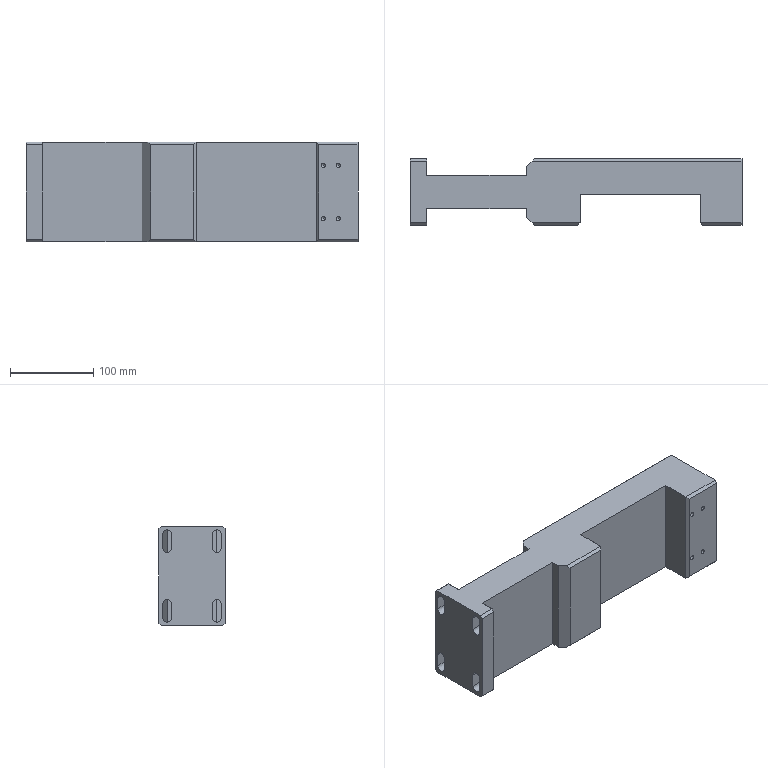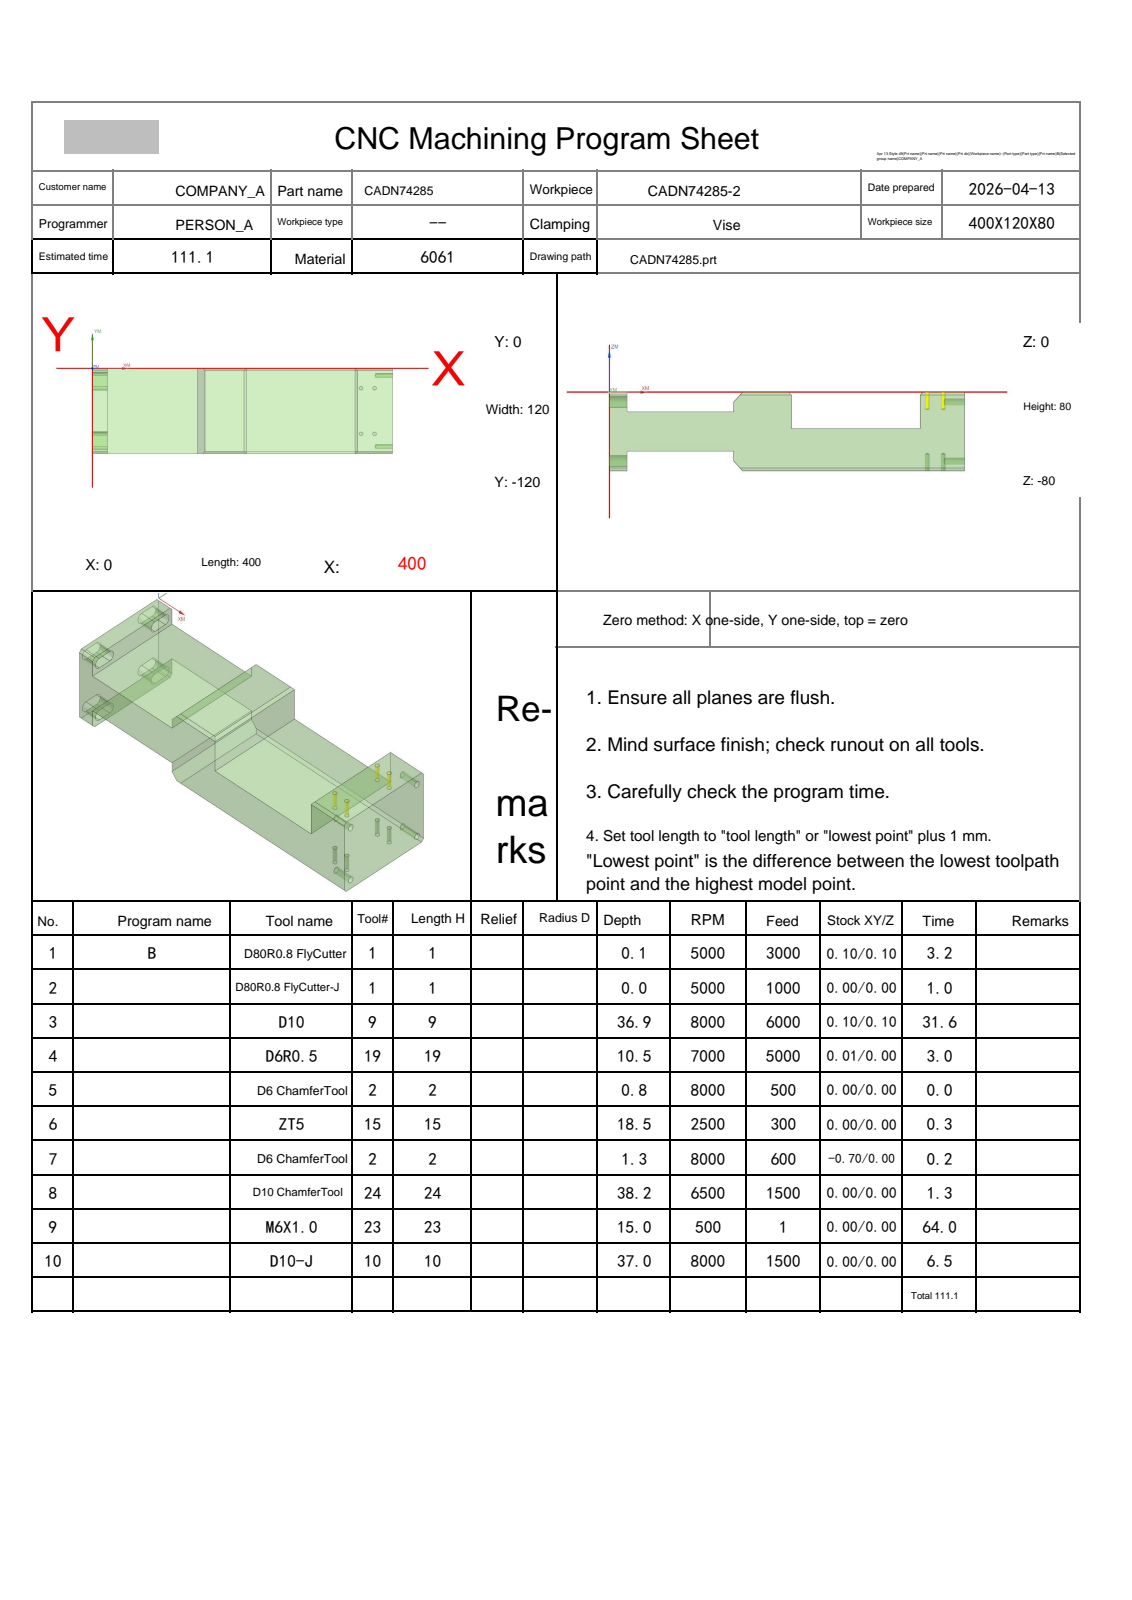NC program | NX | posted by the shop | part box 400 x 80 x 120 mm
Lines 148 to 1262 of 11018:
N3 T09 M06
(D10  D=10. R=0. H=09 ce=0.10 di=0.10)
G00 G90 G54 X281.7 Y-134.5 M03 S8000
G43 H09 Z14.8
M08
Z.404
G01 Z-.796 F6000.
Y-127.08
G03 X274.7 Y-120.08 I-7. J0.0
G01 X210.176
G02 X209.144 Y-123. I-5.292 J.229
G01 X206.806
G02 X202.867 Y-124.337 I-3.939 J5.133
G01 X149.133
G02 X145.194 Y-123. I0.0 J6.471
G01 X142.86
G02 X142.513 Y-122.469 I4.246 J3.15
G01 X142.281 Y-122.023
X142.117 Y-121.559
X141.891 Y-120.662
X141.789 Y-120.08
X135.073
X135.144 Y-120.637
X135.177 Y-120.857
X135.243 Y-121.187
X135.332 Y-121.516
X135.446 Y-121.845
X135.586 Y-122.175
X135.756 Y-122.504
X135.888 Y-122.723
X136.081 Y-123.
X135.852
G02 X134.823 Y-120.08 I4.186 J3.116
G01 X26.095
X25.178
G02 X24.433 Y-122.58 I-5.192 J.186
X24.15 Y-123. I-4.447 J2.686
G01 X23.935
G02 X20. Y-124.337 I-3.956 J5.184
G01 X.08
Y-123.
X.026
Y-124.337
X0.0
Y-123.
X-.08
Y-122.937
X-.001
X0.0 Y-122.938
X.026 Y-122.937
X.027
X.08 Y-122.938
X20. Y-122.937
G03 X25.1 Y-117.817 I-.021 J5.121
G01 Y-117.796
Y-2.204
Y-2.183
G03 X20. Y2.937 I-5.121 J0.0
G01 X.08
X-.08
Y3.
X.08
Y4.337
X20.006
G02 X23.935 Y3. I-.026 J-6.521
G01 X24.15
G02 X25.178 Y.08 I-4.164 J-3.106
G01 X134.824
G02 X135.861 Y3. I5.378 J-.266
G01 X136.079
X135.912 Y2.761
X135.787 Y2.557
X135.696 Y2.395
X135.535 Y2.064
X135.405 Y1.736
X135.284 Y1.351
X135.197 Y.967
X135.144 Y.637
X135.077 Y.11
X135.215 Y.08
X138.463
G02 X139.404 Y-.583 I0.0 J-1.
G01 X141.485 Y-6.408
G03 X142.044 Y-6.995 I.941 J.337
G02 X142.663 Y-7.915 I-.381 J-.924
G01 Y-112.085
G02 X141.667 Y-113.08 I-1. J.005
G01 X135.073
X134.952 Y-113.081
X134.823 Y-113.08
X33.095
G02 X32.1 Y-112.085 I.005 J1.
G01 Y-7.915
G02 X33.095 Y-6.92 I1. J-.005
G01 X39.1
X134.468
X138.169
G02 X138.868 Y-7.62 I0.0 J-.7
X138.826 Y-7.859 I-.7 J0.0
G01 X135.722 Y-16.404
G03 X135.663 Y-16.744 I.94 J-.341
G01 Y-105.085
G02 X134.668 Y-106.08 I-1. J.005
G01 X40.095
G02 X39.1 Y-105.085 I.005 J1.
G01 Y-14.915
G02 X40.095 Y-13.92 I1. J-.005
G01 X131.967
G02 X132.567 Y-14.52 I-.001 J-.6
X132.517 Y-14.759 I-.6 J0.0
G01 X128.745 Y-23.438
G03 X128.663 Y-23.836 I.917 J-.398
G01 Y-98.086
G02 X127.668 Y-99.08 I-1. J.006
G01 X47.094
G02 X46.1 Y-98.086 I.006 J1.
G01 Y-21.914
G02 X47.094 Y-20.92 I1. J-.006
G01 X125.022
G02 X125.622 Y-21.52 I-.001 J-.6
X125.571 Y-21.761 I-.6 J0.0
G01 X121.747 Y-30.442
G03 X121.663 Y-30.844 I.915 J-.403
G01 Y-91.086
G02 X120.668 Y-92.08 I-1. J.006
G01 X54.094
G02 X53.1 Y-91.086 I.006 J1.
G01 Y-28.914
G02 X54.094 Y-27.92 I1. J-.006
G01 X118.027
G02 X118.627 Y-28.52 I0.0 J-.6
X118.576 Y-28.762 I-.6 J0.0
G01 X114.747 Y-37.442
G03 X114.663 Y-37.845 I.915 J-.403
G01 Y-84.086
G02 X113.668 Y-85.08 I-1. J.006
G01 X61.094
G02 X60.1 Y-84.086 I.006 J1.
G01 Y-35.914
G02 X61.094 Y-34.92 I1. J-.006
G01 X111.028
G02 X111.627 Y-35.52 I0.0 J-.6
X111.577 Y-35.762 I-.6 J0.0
G01 X107.747 Y-44.442
G03 X107.663 Y-44.845 I.915 J-.403
G01 Y-77.086
G02 X106.668 Y-78.08 I-1. J.006
G01 X68.094
G02 X67.1 Y-77.086 I.006 J1.
G01 Y-42.914
G02 X68.094 Y-41.92 I1. J-.006
G01 X104.028
G02 X104.628 Y-42.52 I0.0 J-.6
X104.577 Y-42.762 I-.6 J0.0
G01 X100.747 Y-51.442
G03 X100.663 Y-51.845 I.915 J-.403
G01 Y-70.086
G02 X99.669 Y-71.08 I-1. J.006
G01 X75.094
G02 X74.1 Y-70.086 I.006 J1.
G01 Y-49.914
G02 X75.094 Y-48.92 I1. J-.006
G01 X97.028
G02 X97.628 Y-49.52 I0.0 J-.6
X97.577 Y-49.762 I-.6 J0.0
G01 X93.748 Y-58.442
G03 X93.663 Y-58.845 I.915 J-.403
G01 Y-63.086
G02 X92.669 Y-64.08 I-1. J.006
G01 X82.094
G02 X81.1 Y-63.086 I.006 J1.
G01 Y-56.914
G02 X82.094 Y-55.92 I1. J-.006
G01 X90.629
G03 X91.208 Y-55.735 I-.001 J1.
G01 X100.302 Y-49.261
X100.428 Y-49.154
X107.37 Y-42.213
X114.37 Y-35.213
X121.369 Y-28.212
X128.364 Y-21.21
X128.367 Y-21.207
X135.301 Y-14.189
X135.341 Y-14.146
X141.451 Y-7.167
G03 X141.695 Y-6.593 I-.753 J.658
G01 X142.433 Y2.115
G02 X142.544 Y2.477 I.897 J-.077
X142.877 Y3. I4.8 J-2.683
G01 X145.194
G02 X149.133 Y4.337 I3.939 J-5.134
G01 X202.867
G02 X206.806 Y3. I0.0 J-6.471
G01 X209.099
G02 X210.187 Y.08 I-4.43 J-3.314
G01 X344.823
G02 X345.85 Y3. I5.198 J-.188
G01 X348.194
G02 X352.133 Y4.337 I3.939 J-5.133
G01 X399.92
Y3.
X400.08
Y2.937
X399.92 Y2.938
X352.133 Y2.937
G03 X347.063 Y-2.133 I0.0 J-5.071
G01 Y-117.867
G03 X352.133 Y-122.937 I5.071 J0.0
G01 X400.
X400.001
X400.08
Y-123.
X400.
Y-124.337
X352.133
G02 X348.194 Y-123. I0.0 J6.471
G01 X345.865
G02 X344.824 Y-120.08 I4.252 J3.162
G01 X277.714
G02 X276.901 Y-119.662 I.001 J1.
G01 X272.499 Y-113.498
G03 X271.686 Y-113.08 I-.813 J-.582
G01 X210.333
G02 X209.337 Y-112.085 I.005 J1.
G01 Y-8.407
G03 X208.893 Y-7.704 I-.779 J-.001
G01 X208.537 Y-7.536
X208.357 Y-7.495
G03 X207.937 Y-7.915 I0.0 J-.42
G01 Y-117.867
G02 X202.867 Y-122.937 I-5.071 J0.0
G01 X149.133
G02 X144.063 Y-117.867 I0.0 J5.071
G01 Y-2.133
G02 X149.133 Y2.937 I5.071 J0.0
G01 X202.867
G02 X207.937 Y-2.133 I0.0 J-5.071
G01 Y-7.915
G03 X208.357 Y-8.335 I.42 J0.0
G01 X208.537 Y-8.295
X209.136 Y-8.011
G03 X209.356 Y-7.727 I-.172 J.361
G02 X210.333 Y-6.92 I.981 J-.193
G01 X339.067
G02 X340.063 Y-7.915 I-.005 J-1.
G01 Y-112.085
G02 X339.067 Y-113.08 I-1. J.005
G01 X277.714
G02 X276.901 Y-112.662 I.001 J1.
G01 X272.499 Y-106.498
G03 X271.686 Y-106.08 I-.813 J-.582
G01 X217.332
G02 X216.337 Y-105.085 I.005 J1.
G01 Y-14.915
G02 X217.332 Y-13.92 I1. J-.005
G01 X332.068
G02 X333.063 Y-14.915 I-.005 J-1.
G01 Y-105.085
G02 X332.068 Y-106.08 I-1. J.005
G01 X277.714
G02 X276.901 Y-105.662 I.001 J1.
G01 X272.499 Y-99.498
G03 X271.686 Y-99.08 I-.813 J-.582
G01 X224.332
G02 X223.337 Y-98.086 I.006 J1.
G01 Y-21.914
G02 X224.332 Y-20.92 I1. J-.006
G01 X325.068
G02 X326.063 Y-21.914 I-.006 J-1.
G01 Y-98.086
G02 X325.068 Y-99.08 I-1. J.006
G01 X277.714
G02 X276.901 Y-98.662 I.001 J1.
G01 X272.499 Y-92.498
G03 X271.686 Y-92.08 I-.813 J-.582
G01 X231.332
G02 X230.337 Y-91.086 I.006 J1.
G01 Y-28.914
G02 X231.332 Y-27.92 I1. J-.006
G01 X318.068
G02 X319.063 Y-28.914 I-.006 J-1.
G01 Y-91.086
G02 X318.068 Y-92.08 I-1. J.006
G01 X277.714
G02 X276.901 Y-91.662 I.001 J1.
G01 X272.499 Y-85.498
G03 X271.686 Y-85.08 I-.813 J-.582
G01 X238.331
G02 X237.337 Y-84.086 I.006 J1.
G01 Y-35.914
G02 X238.331 Y-34.92 I1. J-.006
G01 X311.069
G02 X312.063 Y-35.914 I-.006 J-1.
G01 Y-84.086
G02 X311.069 Y-85.08 I-1. J.006
G01 X277.714
G02 X276.901 Y-84.662 I0.0 J1.
G01 X272.499 Y-78.498
G03 X271.686 Y-78.08 I-.813 J-.582
G01 X245.331
G02 X244.337 Y-77.086 I.006 J1.
G01 Y-42.914
G02 X245.331 Y-41.92 I1. J-.006
G01 X304.069
G02 X305.063 Y-42.914 I-.006 J-1.
G01 Y-77.086
G02 X304.069 Y-78.08 I-1. J.006
G01 X277.714
G02 X276.901 Y-77.662 I0.0 J1.
G01 X272.499 Y-71.498
G03 X271.686 Y-71.08 I-.814 J-.582
G01 X252.331
G02 X251.337 Y-70.086 I.006 J1.
G01 Y-49.914
G02 X252.331 Y-48.92 I1. J-.006
G01 X297.069
G02 X298.063 Y-49.914 I-.006 J-1.
G01 Y-70.086
G02 X297.069 Y-71.08 I-1. J.006
G01 X277.714
G02 X276.901 Y-70.662 I0.0 J1.
G01 X272.499 Y-64.498
G03 X271.686 Y-64.08 I-.814 J-.582
G01 X259.331
G02 X258.337 Y-63.086 I.006 J1.
G01 Y-56.914
G02 X259.331 Y-55.92 I1. J-.006
G01 X290.069
G02 X291.063 Y-56.914 I-.006 J-1.
G01 Y-63.086
G02 X290.069 Y-64.08 I-1. J.006
G01 X274.7
X274.2
G03 X267.2 Y-71.08 I0.0 J-7.
G01 Z.404
G00 Z3.
G01 X281.7 Y-134.5
G00 Z-.392
G01 Z-1.592
Y-127.08
G03 X274.7 Y-120.08 I-7. J0.0
G01 X210.176
G02 X204.915 Y-125.148 I-5.292 J.229
G01 X147.717 Y-125.151
X146.821 Y-125.129
G02 X142.513 Y-122.469 I.285 J5.279
G01 X142.281 Y-122.023
X142.117 Y-121.559
X141.891 Y-120.662
X141.789 Y-120.08
X135.073
X135.144 Y-120.637
X135.177 Y-120.857
X135.243 Y-121.187
X135.332 Y-121.516
X135.446 Y-121.845
X135.586 Y-122.175
X135.756 Y-122.504
X135.888 Y-122.723
X136.117 Y-123.053
X136.289 Y-123.267
X136.502 Y-123.499
X136.565 Y-123.556
X136.501 Y-123.612
X136.446 Y-123.676
X136.388 Y-123.614
G02 X134.823 Y-120.08 I3.65 J3.73
G01 X25.178
G02 X23.55 Y-123.674 I-5.192 J.186
X19.92 Y-125.148 I-3.664 J3.815
G01 X0.0 Y-125.151
X-.085 Y-125.156
X-.08 Y-125.071
Y-123.733
X0.0
X20.
G03 X25.1 Y-118.613 I-.021 J5.121
G01 Y-118.592
Y-1.408
Y-1.387
G03 X20. Y3.733 I-5.121 J0.0
G01 X.08
X.002
X0.0
X-.08
Y5.071
X-.085 Y5.156
X0.0 Y5.151
X19.92 Y5.142
G02 X23.55 Y3.674 I-.035 J-5.308
X25.178 Y.08 I-3.564 J-3.78
G01 X134.824
G02 X136.437 Y3.664 I5.378 J-.266
G01 X136.498 Y3.727
X136.553 Y3.66
X136.615 Y3.603
X136.552 Y3.548
X136.453 Y3.45
X136.293 Y3.272
X136.164 Y3.113
X136.036 Y2.943
X135.912 Y2.761
X135.787 Y2.557
X135.696 Y2.395
X135.535 Y2.064
X135.405 Y1.736
X135.284 Y1.351
X135.197 Y.967
X135.144 Y.637
X135.077 Y.11
X135.215 Y.08
X137.666
G02 X138.607 Y-.583 I0.0 J-1.
G01 X140.688 Y-6.408
G03 X141.247 Y-6.995 I.941 J.337
G02 X141.867 Y-7.916 I-.381 J-.925
G01 Y-112.084
G02 X140.871 Y-113.08 I-1. J.004
G01 X135.073
X134.823
X33.096
G02 X32.1 Y-112.084 I.004 J1.
G01 Y-7.916
G02 X33.096 Y-6.92 I1. J-.004
G01 X39.1
X134.468
X137.372
G02 X138.072 Y-7.62 I0.0 J-.7
X138.03 Y-7.859 I-.7 J0.0
G01 X134.926 Y-16.404
G03 X134.867 Y-16.744 I.94 J-.341
G01 Y-105.085
G02 X133.871 Y-106.08 I-1. J.005
G01 X40.095
G02 X39.1 Y-105.085 I.005 J1.
G01 Y-14.915
G02 X40.095 Y-13.92 I1. J-.005
G01 X131.171
G02 X131.771 Y-14.52 I-.001 J-.6
X131.721 Y-14.759 I-.6 J0.0
G01 X127.949 Y-23.438
G03 X127.867 Y-23.836 I.917 J-.398
G01 Y-98.085
G02 X126.871 Y-99.08 I-1. J.005
G01 X47.095
G02 X46.1 Y-98.085 I.005 J1.
G01 Y-21.915
G02 X47.095 Y-20.92 I1. J-.005
G01 X124.226
G02 X124.826 Y-21.52 I0.0 J-.6
X124.775 Y-21.761 I-.6 J0.0
G01 X120.951 Y-30.442
G03 X120.867 Y-30.844 I.915 J-.403
G01 Y-91.085
G02 X119.871 Y-92.08 I-1. J.005
G01 X54.095
G02 X53.1 Y-91.085 I.005 J1.
G01 Y-28.915
G02 X54.095 Y-27.92 I1. J-.005
G01 X117.231
G02 X117.831 Y-28.52 I0.0 J-.6
X117.78 Y-28.762 I-.6 J0.0
G01 X113.951 Y-37.442
G03 X113.867 Y-37.845 I.915 J-.403
G01 Y-84.085
G02 X112.872 Y-85.08 I-1. J.005
G01 X61.095
G02 X60.1 Y-84.085 I.005 J1.
G01 Y-35.915
G02 X61.095 Y-34.92 I1. J-.005
G01 X110.232
G02 X110.831 Y-35.52 I0.0 J-.6
X110.781 Y-35.762 I-.6 J0.0
G01 X106.951 Y-44.442
G03 X106.867 Y-44.845 I.915 J-.403
G01 Y-77.085
G02 X105.872 Y-78.08 I-1. J.005
G01 X68.095
G02 X67.1 Y-77.085 I.005 J1.
G01 Y-42.915
G02 X68.095 Y-41.92 I1. J-.005
G01 X103.232
G02 X103.832 Y-42.52 I0.0 J-.6
X103.781 Y-42.762 I-.6 J0.0
G01 X99.951 Y-51.442
G03 X99.867 Y-51.845 I.915 J-.403
G01 Y-70.085
G02 X98.872 Y-71.08 I-1. J.005
G01 X75.095
G02 X74.1 Y-70.085 I.005 J1.
G01 Y-49.915
G02 X75.095 Y-48.92 I1. J-.005
G01 X96.232
G02 X96.832 Y-49.52 I0.0 J-.6
X96.781 Y-49.762 I-.6 J0.0
G01 X92.952 Y-58.442
G03 X92.867 Y-58.845 I.915 J-.403
G01 Y-63.085
G02 X91.872 Y-64.08 I-1. J.005
G01 X82.095
G02 X81.1 Y-63.085 I.005 J1.
G01 Y-56.915
G02 X82.095 Y-55.92 I1. J-.005
G01 X89.833
G03 X90.412 Y-55.735 I-.001 J1.
G01 X99.506 Y-49.261
X99.632 Y-49.154
X106.574 Y-42.213
X113.574 Y-35.213
X120.573 Y-28.212
X127.568 Y-21.21
X127.571 Y-21.207
X134.505 Y-14.189
X134.545 Y-14.145
X140.678 Y-7.14
G03 X140.914 Y-6.63 I-.753 J.658
G01 X142.124 Y1.473
X142.173 Y1.664
G02 X144.103 Y4.236 I5.171 J-1.871
X147.426 Y5.157 I3.324 J-5.531
X147.721 Y5.151 I0.0 J-6.453
G01 X204.923 Y5.142
X205.829 Y5.057
X206.733 Y4.819
G02 X210.187 Y.08 I-2.064 J-5.133
G01 X344.823
G02 X346.473 Y3.695 I5.198 J-.188
X350.341 Y5.156 I3.868 J-4.391
X350.59 Y5.151 I0.0 J-5.852
G01 X400.
X400.085 Y5.156
X400.08 Y5.071
Y3.733
X400.
X351.337
G03 X346.266 Y-1.419 I.082 J-5.152
G01 X346.267 Y-1.501
Y-118.663
G03 X351.337 Y-123.733 I5.071 J0.0
G01 X399.973
X400.08
Y-124.215
Y-125.071
X400.085 Y-125.156
X400. Y-125.151
X350.585
X349.688 Y-125.119
G02 X344.824 Y-120.08 I.429 J5.281
G01 X277.714
G02 X276.901 Y-119.662 I.001 J1.
G01 X272.499 Y-113.498
G03 X271.686 Y-113.08 I-.813 J-.582
G01 X211.13
G02 X210.133 Y-112.084 I.004 J1.
G01 Y-8.408
G03 X209.689 Y-7.705 I-.779 J-.001
G01 X209.333 Y-7.537
X209.153 Y-7.496
G03 X208.733 Y-7.916 I0.0 J-.42
G01 Y-118.663
G02 X203.663 Y-123.733 I-5.071 J0.0
G01 X148.337
G02 X143.267 Y-118.663 I0.0 J5.071
G01 Y-1.337
G02 X148.337 Y3.733 I5.071 J0.0
G01 X203.663
G02 X208.733 Y-1.337 I0.0 J-5.071
G01 Y-7.916
G03 X209.153 Y-8.336 I.42 J0.0
G01 X209.333 Y-8.296
X209.931 Y-8.012
G03 X210.152 Y-7.728 I-.172 J.361
G02 X211.129 Y-6.92 I.981 J-.192
G01 X338.271
G02 X339.267 Y-7.916 I-.004 J-1.
G01 Y-112.084
G02 X338.27 Y-113.08 I-1. J.004
G01 X277.714
G02 X276.901 Y-112.662 I.001 J1.
G01 X272.499 Y-106.498
G03 X271.686 Y-106.08 I-.813 J-.582
G01 X218.129
G02 X217.133 Y-105.085 I.005 J1.
G01 Y-14.915
G02 X218.129 Y-13.92 I1. J-.005
G01 X331.271
G02 X332.267 Y-14.915 I-.005 J-1.
G01 Y-105.085
G02 X331.271 Y-106.08 I-1. J.005
G01 X277.714
G02 X276.901 Y-105.662 I.001 J1.
G01 X272.499 Y-99.498
G03 X271.686 Y-99.08 I-.813 J-.582
G01 X225.129
G02 X224.133 Y-98.085 I.005 J1.
G01 Y-21.915
G02 X225.129 Y-20.92 I1. J-.005
G01 X324.271
G02 X325.267 Y-21.915 I-.005 J-1.
G01 Y-98.085
G02 X324.271 Y-99.08 I-1. J.005
G01 X277.714
G02 X276.901 Y-98.662 I.001 J1.
G01 X272.499 Y-92.498
G03 X271.686 Y-92.08 I-.813 J-.582
G01 X232.128
G02 X231.133 Y-91.085 I.005 J1.
G01 Y-28.915
G02 X232.128 Y-27.92 I1. J-.005
G01 X317.272
G02 X318.267 Y-28.915 I-.005 J-1.
G01 Y-91.085
G02 X317.272 Y-92.08 I-1. J.005
G01 X277.714
G02 X276.901 Y-91.662 I.001 J1.
G01 X272.499 Y-85.498
G03 X271.686 Y-85.08 I-.813 J-.582
G01 X239.128
G02 X238.133 Y-84.085 I.005 J1.
G01 Y-35.915
G02 X239.128 Y-34.92 I1. J-.005
G01 X310.272
G02 X311.267 Y-35.915 I-.005 J-1.
G01 Y-84.085
G02 X310.272 Y-85.08 I-1. J.005
G01 X277.714
G02 X276.901 Y-84.662 I0.0 J1.
G01 X272.499 Y-78.498
G03 X271.686 Y-78.08 I-.813 J-.582
G01 X246.128
G02 X245.133 Y-77.085 I.005 J1.
G01 Y-42.915
G02 X246.128 Y-41.92 I1. J-.005
G01 X303.272
G02 X304.267 Y-42.915 I-.005 J-1.
G01 Y-77.085
G02 X303.272 Y-78.08 I-1. J.005
G01 X277.714
G02 X276.901 Y-77.662 I0.0 J1.
G01 X272.499 Y-71.498
G03 X271.686 Y-71.08 I-.813 J-.582
G01 X253.128
G02 X252.133 Y-70.085 I.005 J1.
G01 Y-49.915
G02 X253.128 Y-48.92 I1. J-.005
G01 X296.272
G02 X297.267 Y-49.915 I-.005 J-1.
G01 Y-70.085
G02 X296.272 Y-71.08 I-1. J.005
G01 X277.714
G02 X276.901 Y-70.662 I0.0 J1.
G01 X272.499 Y-64.498
G03 X271.686 Y-64.08 I-.814 J-.582
G01 X260.128
G02 X259.133 Y-63.086 I.006 J1.
G01 Y-56.914
G02 X260.128 Y-55.92 I1. J-.006
G01 X289.272
G02 X290.267 Y-56.914 I-.006 J-1.
G01 Y-63.086
G02 X289.272 Y-64.08 I-1. J.006
G01 X274.7
X274.2
G03 X267.2 Y-71.08 I0.0 J-7.
G01 Z-.392
G00 Z3.
G01 X281.7 Y-134.5
G00 Z-1.188
G01 Z-2.388
Y-127.08
G03 X274.7 Y-120.08 I-7. J0.0
G01 X210.176
G02 X204.915 Y-125.148 I-5.292 J.229
G01 X147.717 Y-125.151
X146.821 Y-125.129
G02 X142.513 Y-122.469 I.285 J5.279
G01 X142.281 Y-122.023
X142.117 Y-121.559
X141.891 Y-120.662
X141.789 Y-120.08
X135.073
X135.144 Y-120.637
X135.177 Y-120.857
X135.243 Y-121.187
X135.332 Y-121.516
X135.446 Y-121.845
X135.586 Y-122.175
X135.756 Y-122.504
X135.888 Y-122.723
X136.117 Y-123.053
X136.289 Y-123.267
X136.502 Y-123.499
X136.565 Y-123.556
X136.501 Y-123.612
X136.446 Y-123.676
X136.388 Y-123.614
G02 X134.823 Y-120.08 I3.65 J3.73
G01 X25.178
G02 X23.55 Y-123.674 I-5.192 J.186
X19.92 Y-125.148 I-3.664 J3.815
G01 X0.0 Y-125.151
X-.085 Y-125.156
X-.08 Y-125.071
Y-124.534
X0.0
X.074
X.08
X.259 Y-124.529
X20.
G03 X25.1 Y-119.388 I-.048 J5.147
G01 Y-.612
G03 X20. Y4.529 I-5.148 J-.006
G01 X.08
X.01
X0.0
X-.08
Y5.071
X-.085 Y5.156
X0.0 Y5.151
X19.92 Y5.142
G02 X23.55 Y3.674 I-.035 J-5.308
X25.178 Y.08 I-3.564 J-3.78
G01 X134.824
G02 X136.437 Y3.664 I5.378 J-.266
G01 X136.498 Y3.727
X136.553 Y3.66
X136.615 Y3.603
X136.552 Y3.548
X136.453 Y3.45
X136.293 Y3.272
X136.164 Y3.113
X136.036 Y2.943
X135.912 Y2.761
X135.787 Y2.557
X135.696 Y2.395
X135.535 Y2.064
X135.405 Y1.736
X135.284 Y1.351
X135.197 Y.967
X135.144 Y.637
X135.077 Y.11
X135.215 Y.08
X136.87
G02 X137.812 Y-.583 I0.0 J-1.
G01 X139.892 Y-6.408
G03 X140.452 Y-6.995 I.941 J.337
G02 X141.071 Y-7.916 I-.381 J-.925
G01 Y-112.084
G02 X140.075 Y-113.08 I-1. J.004
G01 X135.073
X134.952 Y-113.081
X134.823 Y-113.08
X33.096
G02 X32.1 Y-112.084 I.004 J1.
G01 Y-7.916
G02 X33.096 Y-6.92 I1. J-.004
G01 X134.468
X136.576
G02 X137.276 Y-7.62 I0.0 J-.7
X137.234 Y-7.859 I-.7 J0.0
G01 X134.13 Y-16.404
G03 X134.071 Y-16.744 I.94 J-.341
G01 Y-105.085
G02 X133.076 Y-106.08 I-1. J.005
G01 X40.095
G02 X39.1 Y-105.085 I.005 J1.
G01 Y-14.915
G02 X40.095 Y-13.92 I1. J-.005
G01 X130.375
G02 X130.975 Y-14.52 I-.001 J-.6
X130.925 Y-14.759 I-.6 J0.0
G01 X127.153 Y-23.438
G03 X127.071 Y-23.836 I.917 J-.398
G01 Y-98.085
G02 X126.076 Y-99.08 I-1. J.005
G01 X47.095
G02 X46.1 Y-98.085 I.005 J1.
G01 Y-21.915
G02 X47.095 Y-20.92 I1. J-.005
G01 X123.43
G02 X124.03 Y-21.52 I-.001 J-.6
X123.979 Y-21.761 I-.6 J0.0
G01 X120.155 Y-30.442
G03 X120.071 Y-30.844 I.915 J-.403
G01 Y-91.085
G02 X119.076 Y-92.08 I-1. J.005
G01 X54.095
G02 X53.1 Y-91.085 I.005 J1.
G01 Y-28.915
G02 X54.095 Y-27.92 I1. J-.005
G01 X116.435
G02 X117.035 Y-28.52 I0.0 J-.6
X116.984 Y-28.762 I-.6 J0.0
G01 X113.155 Y-37.442
G03 X113.071 Y-37.845 I.915 J-.403
G01 Y-84.085
G02 X112.076 Y-85.08 I-1. J.005
G01 X61.095
G02 X60.1 Y-84.085 I.005 J1.
G01 Y-35.915
G02 X61.095 Y-34.92 I1. J-.005
G01 X109.436
G02 X110.035 Y-35.52 I0.0 J-.6
X109.985 Y-35.762 I-.6 J0.0
G01 X106.155 Y-44.442
G03 X106.071 Y-44.845 I.915 J-.403
G01 Y-77.086
G02 X105.076 Y-78.08 I-1. J.006
G01 X68.094
G02 X67.1 Y-77.086 I.006 J1.
G01 Y-42.914
G02 X68.094 Y-41.92 I1. J-.006
G01 X102.436
G02 X103.036 Y-42.52 I0.0 J-.6
X102.985 Y-42.762 I-.6 J0.0
G01 X99.155 Y-51.442
G03 X99.071 Y-51.845 I.915 J-.403
G01 Y-70.086
G02 X98.076 Y-71.08 I-1. J.006
G01 X75.094
G02 X74.1 Y-70.086 I.006 J1.
G01 Y-49.914
G02 X75.094 Y-48.92 I1. J-.006
G01 X95.436
G02 X96.036 Y-49.52 I0.0 J-.6
X95.985 Y-49.762 I-.6 J0.0
G01 X92.156 Y-58.442
G03 X92.071 Y-58.845 I.915 J-.403
G01 Y-63.086
G02 X91.076 Y-64.08 I-1. J.006
G01 X82.094
G02 X81.1 Y-63.086 I.006 J1.
G01 Y-56.914
G02 X82.094 Y-55.92 I1. J-.006
G01 X89.037
G03 X89.616 Y-55.735 I-.001 J1.
G01 X98.71 Y-49.261
X98.836 Y-49.154
X105.778 Y-42.213
X112.778 Y-35.213
X119.777 Y-28.212
X126.772 Y-21.21
X126.775 Y-21.207
X133.709 Y-14.189
X133.749 Y-14.145
X139.917 Y-7.1
G03 X140.134 Y-6.688 I-.753 J.658
G01 X141.829 Y-.011
X141.858 Y.166
G02 X144.103 Y4.236 I5.486 J-.373
X147.426 Y5.157 I3.324 J-5.531
X147.721 Y5.151 I0.0 J-6.453
G01 X204.923 Y5.142
X205.829 Y5.057
X206.733 Y4.819
G02 X210.187 Y.08 I-2.064 J-5.133
G01 X344.823
G02 X346.473 Y3.695 I5.198 J-.188
X350.341 Y5.156 I3.868 J-4.391
X350.59 Y5.151 I0.0 J-5.852
G01 X400.
X400.085 Y5.156
X400.08 Y5.071
Y4.534
X400.
X399.955
G03 X399.742 Y4.529 I0.0 J-5.145
G01 X350.541
G03 X345.471 Y-.541 I0.0 J-5.071
G01 Y-119.459
G03 X350.541 Y-124.529 I5.071 J0.0
G01 X399.742
G03 X399.955 Y-124.534 I.214 J5.141
G01 X400.
X400.08
Y-125.071
X400.085 Y-125.156
X400. Y-125.151
X350.585
X349.688 Y-125.119
G02 X344.824 Y-120.08 I.429 J5.281
G01 X277.714
G02 X276.901 Y-119.662 I.001 J1.
G01 X272.499 Y-113.498
G03 X271.686 Y-113.08 I-.813 J-.582
G01 X211.925
G02 X210.929 Y-112.084 I.004 J1.
G01 Y-8.408
G03 X210.485 Y-7.705 I-.779 J-.001
G01 X210.129 Y-7.536
X209.949 Y-7.496
G03 X209.529 Y-7.916 I0.0 J-.42
G01 Y-119.459
G02 X204.459 Y-124.529 I-5.071 J0.0
G01 X147.541
G02 X142.471 Y-119.459 I0.0 J5.071
G01 Y-.541
G02 X147.541 Y4.529 I5.071 J0.0
G01 X204.459
G02 X209.529 Y-.541 I0.0 J-5.071
G01 Y-7.916
G03 X209.949 Y-8.336 I.42 J0.0
G01 X210.129 Y-8.295
X210.728 Y-8.011
G03 X210.948 Y-7.728 I-.172 J.361
G02 X211.925 Y-6.92 I.981 J-.192
G01 X337.475
G02 X338.471 Y-7.916 I-.004 J-1.
G01 Y-112.084
G02 X337.475 Y-113.08 I-1. J.004
G01 X277.714
G02 X276.901 Y-112.662 I.001 J1.
G01 X272.499 Y-106.498
G03 X271.686 Y-106.08 I-.813 J-.582
G01 X218.924
G02 X217.929 Y-105.085 I.005 J1.
G01 Y-14.915
G02 X218.924 Y-13.92 I1. J-.005
G01 X330.476
G02 X331.471 Y-14.915 I-.005 J-1.
G01 Y-105.085
G02 X330.476 Y-106.08 I-1. J.005
G01 X277.714
G02 X276.901 Y-105.662 I.001 J1.
G01 X272.499 Y-99.498
G03 X271.686 Y-99.08 I-.813 J-.582
G01 X225.924
G02 X224.929 Y-98.085 I.005 J1.
G01 Y-21.915
G02 X225.924 Y-20.92 I1. J-.005
G01 X323.476
G02 X324.471 Y-21.915 I-.005 J-1.
G01 Y-98.085
G02 X323.476 Y-99.08 I-1. J.005
G01 X277.714
G02 X276.901 Y-98.662 I.001 J1.
G01 X272.499 Y-92.498
G03 X271.686 Y-92.08 I-.813 J-.582
G01 X232.924
G02 X231.929 Y-91.085 I.005 J1.
G01 Y-28.915
G02 X232.924 Y-27.92 I1. J-.005
G01 X316.476
G02 X317.471 Y-28.915 I-.005 J-1.
G01 Y-91.085
G02 X316.476 Y-92.08 I-1. J.005
G01 X277.714
G02 X276.901 Y-91.662 I.001 J1.
G01 X272.499 Y-85.498
G03 X271.686 Y-85.08 I-.813 J-.582
G01 X239.924
G02 X238.929 Y-84.086 I.006 J1.
G01 Y-35.914
G02 X239.924 Y-34.92 I1. J-.006
G01 X309.476
G02 X310.471 Y-35.914 I-.006 J-1.
G01 Y-84.086
G02 X309.476 Y-85.08 I-1. J.006
G01 X277.714
G02 X276.901 Y-84.662 I0.0 J1.
G01 X272.499 Y-78.498
G03 X271.686 Y-78.08 I-.813 J-.582
G01 X246.924
G02 X245.929 Y-77.086 I.006 J1.
G01 Y-42.914
G02 X246.924 Y-41.92 I1. J-.006
G01 X302.476
G02 X303.471 Y-42.914 I-.006 J-1.
G01 Y-77.086
G02 X302.476 Y-78.08 I-1. J.006
G01 X277.714
G02 X276.901 Y-77.662 I0.0 J1.
G01 X272.499 Y-71.498
G03 X271.686 Y-71.08 I-.813 J-.582
G01 X253.924
G02 X252.929 Y-70.086 I.006 J1.
G01 Y-49.914
G02 X253.924 Y-48.92 I1. J-.006
G01 X295.476
G02 X296.471 Y-49.914 I-.006 J-1.
G01 Y-70.086
G02 X295.476 Y-71.08 I-1. J.006
G01 X277.714
G02 X276.901 Y-70.662 I0.0 J1.
G01 X272.499 Y-64.498
G03 X271.686 Y-64.08 I-.814 J-.582
G01 X260.924
G02 X259.929 Y-63.086 I.006 J1.
G01 Y-56.914
G02 X260.924 Y-55.92 I1. J-.006
G01 X288.476
G02 X289.471 Y-56.914 I-.006 J-1.
G01 Y-63.086
G02 X288.476 Y-64.08 I-1. J.006
G01 X274.7
X274.2
G03 X267.2 Y-71.08 I0.0 J-7.
G01 Z-1.188
G00 Z3.
G01 X281.7 Y-134.5
G00 Z-1.984
G01 Z-3.184
Y-127.08
G03 X274.7 Y-120.08 I-7. J0.0
G01 X210.176
G02 X208.547 Y-123.678 I-5.292 J.229
G01 X208.491 Y-123.622
X208.606 Y-123.506
G03 X210.1 Y-119.9 I-3.606 J3.606
G01 Y-.1
G03 X208.606 Y3.506 I-5.1 J0.0
G01 X208.507 Y3.606
X208.539 Y3.639
G02 X209.099 Y3. I-3.87 J-3.953
X210.187 Y.08 I-4.43 J-3.314
G01 X344.823
G02 X345.85 Y3. I5.198 J-.188
X346.469 Y3.692 I4.171 J-3.108
G01 X346.524 Y3.636
X346.394 Y3.506
G03 X344.9 Y-.1 I3.606 J-3.606
G01 Y-119.9
G03 X346.394 Y-123.506 I5.1 J0.0
G01 X346.524 Y-123.636
X346.475 Y-123.687
G02 X344.824 Y-120.08 I3.642 J3.849
G01 X277.714
G02 X276.901 Y-119.662 I.001 J1.
G01 X272.499 Y-113.498
G03 X271.686 Y-113.08 I-.813 J-.582
G01 X218.095
G02 X217.1 Y-112.085 I.005 J1.
G01 Y-7.915
G02 X218.095 Y-6.92 I1. J-.005
G01 X336.905
G02 X337.9 Y-7.915 I-.005 J-1.
G01 Y-112.085
G02 X336.905 Y-113.08 I-1. J.005
G01 X277.714
G02 X276.901 Y-112.662 I.001 J1.
G01 X272.499 Y-106.498
G03 X271.686 Y-106.08 I-.813 J-.582
G01 X225.095
G02 X224.1 Y-105.085 I.005 J1.
G01 Y-14.915
G02 X225.095 Y-13.92 I1. J-.005
G01 X329.905
G02 X330.9 Y-14.915 I-.005 J-1.
G01 Y-105.085
G02 X329.905 Y-106.08 I-1. J.005
G01 X277.714
G02 X276.901 Y-105.662 I.001 J1.
G01 X272.499 Y-99.498
G03 X271.686 Y-99.08 I-.813 J-.582
G01 X232.095
G02 X231.1 Y-98.085 I.005 J1.
G01 Y-21.915
G02 X232.095 Y-20.92 I1. J-.005
G01 X322.905
G02 X323.9 Y-21.915 I-.005 J-1.
G01 Y-98.085
G02 X322.905 Y-99.08 I-1. J.005
G01 X277.714
G02 X276.901 Y-98.662 I.001 J1.
G01 X272.499 Y-92.498
G03 X271.686 Y-92.08 I-.813 J-.582
G01 X239.094
G02 X238.1 Y-91.086 I.006 J1.
G01 Y-28.914
G02 X239.094 Y-27.92 I1. J-.006
G01 X315.906
G02 X316.9 Y-28.914 I-.006 J-1.
G01 Y-91.086
G02 X315.906 Y-92.08 I-1. J.006
G01 X277.714
G02 X276.901 Y-91.662 I0.0 J1.
G01 X272.499 Y-85.498
G03 X271.686 Y-85.08 I-.813 J-.582
G01 X246.094
G02 X245.1 Y-84.086 I.006 J1.
G01 Y-35.914
G02 X246.094 Y-34.92 I1. J-.006
G01 X308.906
G02 X309.9 Y-35.914 I-.006 J-1.
G01 Y-84.086
G02 X308.906 Y-85.08 I-1. J.006
G01 X277.714
G02 X276.901 Y-84.662 I0.0 J1.
G01 X272.499 Y-78.498
G03 X271.686 Y-78.08 I-.813 J-.582
G01 X253.094
G02 X252.1 Y-77.086 I.006 J1.
G01 Y-42.914
G02 X253.094 Y-41.92 I1. J-.006
G01 X301.906
G02 X302.9 Y-42.914 I-.006 J-1.
G01 Y-77.086
G02 X301.906 Y-78.08 I-1. J.006
G01 X277.714
G02 X276.901 Y-77.662 I0.0 J1.
G01 X272.499 Y-71.498
G03 X271.686 Y-71.08 I-.814 J-.582
G01 X260.094
G02 X259.1 Y-70.086 I.006 J1.
G01 Y-49.914
G02 X260.094 Y-48.92 I1. J-.006
G01 X294.906
G02 X295.9 Y-49.914 I-.006 J-1.
G01 Y-70.086
G02 X294.906 Y-71.08 I-1. J.006
G01 X277.714
G02 X276.901 Y-70.662 I0.0 J1.
G01 X272.499 Y-64.499
G03 X271.686 Y-64.08 I-.814 J-.581
G01 X267.094